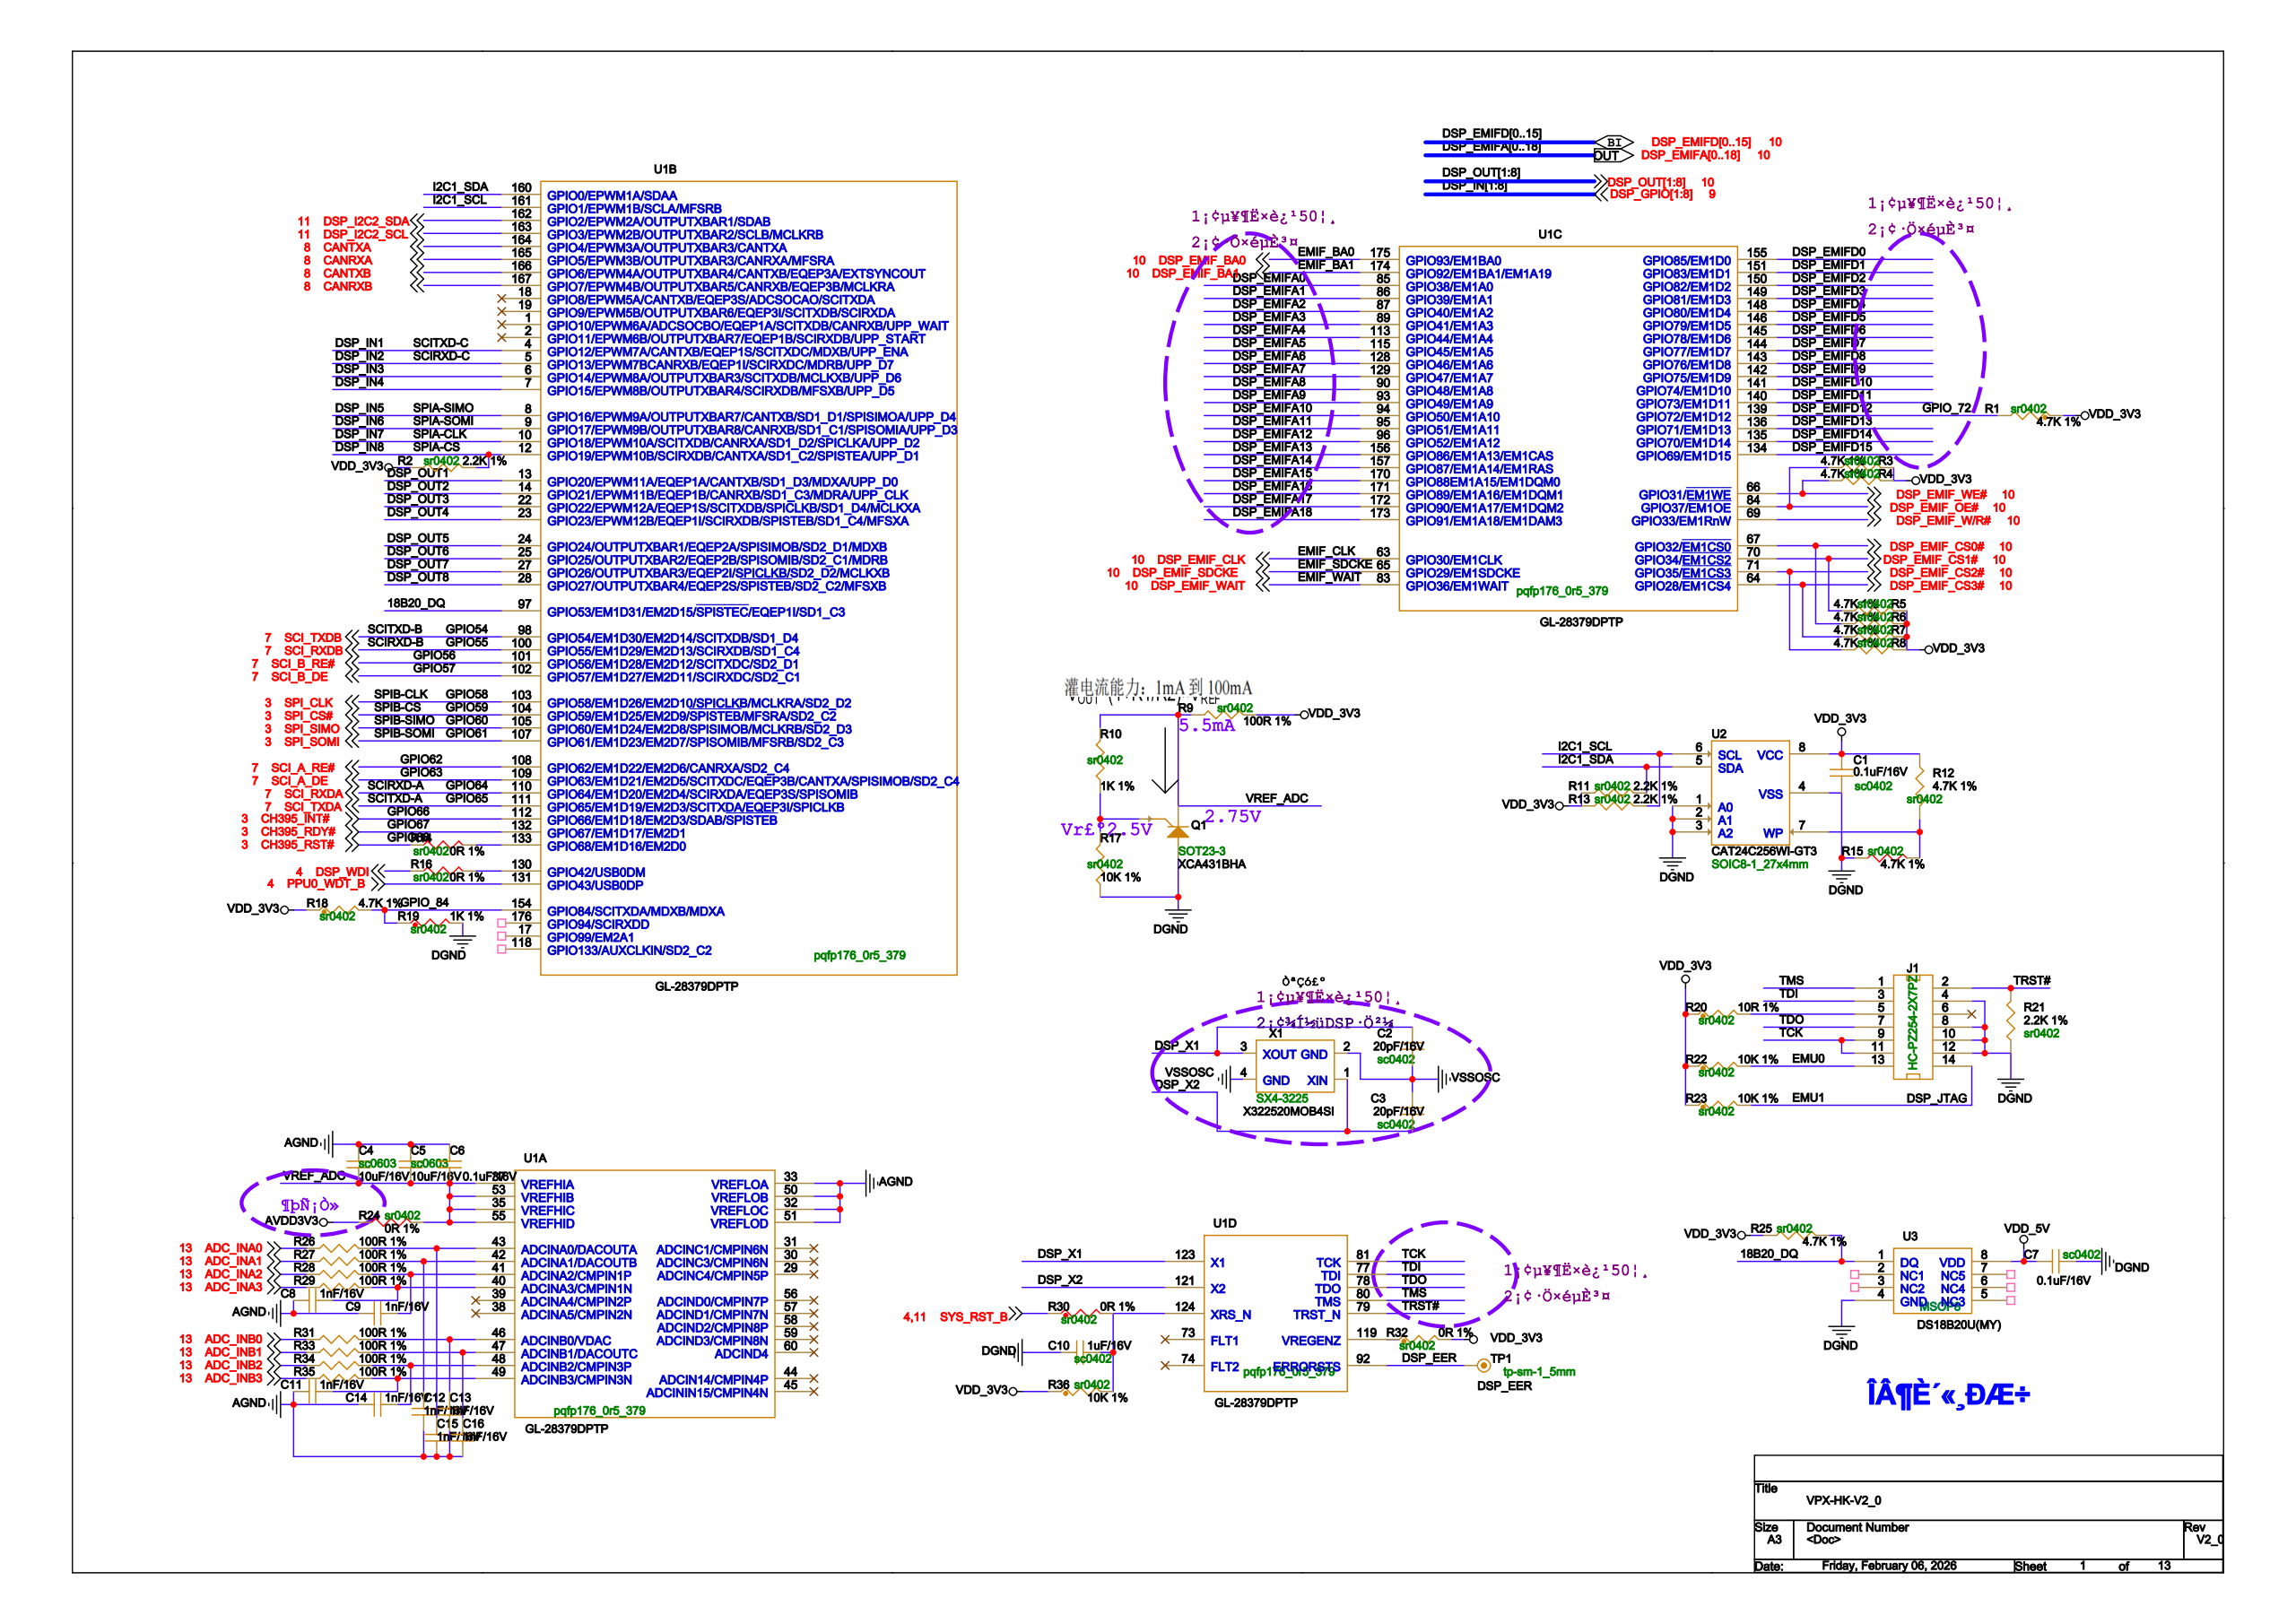Circuit board | Cadence Allegro | 598 parts | 541 nets | one sheet of the schematic
Parts on this sheet (reference | value | footprint):
C2 | 20pF/16V | SC0402
C3 | 20pF/16V | SC0402
C4 | 10uF/16V | SC0603
C5 | 10uF/16V | SC0603
C6 | 0.1uF/16V | SC0402
C8 | 1nF/16V | SC0402
C9 | 1nF/16V | SC0402
C10 | 1uF/16V | SC0402
C11 | 1nF/16V | SC0402
C13 | 1nF/16V | SC0402
C14 | 1nF/16V | SC0402
C15 | 1nF/16V | SC0402
C16 | 1nF/16V | SC0402
J1 | DSP_JTAG | HC-PZ254-2X7PZ
Q1 | XCA431BHA | SOT23-3
R1 | 4.7K 1% | SR0402
R2 | 2.2K 1% | SR0402
R9 | 100R 1% | SR0402
R10 | 1K 1% | SR0402
R11 | 2.2K 1% | SR0402
R12 | 4.7K 1% | SR0402
R13 | 2.2K 1% | SR0402
R14 | 0R 1% | SR0402
R15 | 4.7K 1% | SR0402
R16 | 0R 1% | SR0402
R17 | 10K 1% | SR0402
R18 | 4.7K 1% | SR0402
R19 | 1K 1% | SR0402
R20 | 10R 1% | SR0402
R21 | 2.2K 1% | SR0402
R22 | 10K 1% | SR0402
R23 | 10K 1% | SR0402
R24 | 0R 1% | SR0402
R25 | 4.7K 1% | SR0402
R26 | 100R 1% | SR0402
R27 | 100R 1% | SR0402
R28 | 100R 1% | SR0402
R29 | 100R 1% | SR0402
R30 | 0R 1% | SR0402
R31 | 100R 1% | SR0402
R32 | 0R 1% | SR0402
R33 | 100R 1% | SR0402
R34 | 100R 1% | SR0402
R35 | 100R 1% | SR0402
R36 | 10K 1% | SR0402
TP1 | DSP_EER | TP-SM-1_5MM
U1 | GL-28379DPTP | PQFP176_0R5_379
U2 | CAT24C256WI-GT3 | SOIC8-1_27X4MM
U3 | DS18B20U(MY) | MSOP8
X1 | X322520MOB4SI | SX4-3225
Nets of these parts (net: part-pin ...):
DGND: C10-1 J1-4 J1-8 J1-10 J1-12 Q1-3 R15-2 R17-1 R19-2 R21-2 U2-1 U2-2 U2-3 U2-4 U3-4
VDD_5V: U3-8
DSP_GPIO8: R2-2 U1-12
DSP_OUT7: U1-27
DSP_OUT8: U1-28
DSP_EMIF_CS2#: U1-71
DSP_EMIF_CS3#: U1-64
DSP_EMIF_CS1#: U1-70
DSP_EMIF_CS0#: U1-67
DSP_EMIF_WAIT: U1-83
DSP_EMIF_SDCKE: U1-65
DSP_EMIF_CLK: U1-63
DSP_EMIF_W/R#: U1-69
DSP_EMIF_OE#: U1-84
DSP_EMIF_WE#: U1-66
DSP_EMIF_BA1: U1-174
DSP_EMIF_BA0: U1-175
DSP_EMIFA18: U1-173
DSP_EMIFA17: U1-172
DSP_EMIFA16: U1-171
DSP_EMIFA15: U1-170
DSP_EMIFA14: U1-157
DSP_EMIFA13: U1-156
DSP_EMIFA12: U1-96
DSP_EMIFA11: U1-95
DSP_EMIFA10: U1-94
DSP_EMIFA9: U1-93
DSP_EMIFA8: U1-90
DSP_EMIFA7: U1-129
DSP_EMIFA6: U1-128
DSP_EMIFA5: U1-115
DSP_EMIFA4: U1-113
DSP_EMIFA3: U1-89
DSP_EMIFA2: U1-87
DSP_EMIFA1: U1-86
DSP_EMIFA0: U1-85
DSP_OUT5: U1-24
DSP_OUT6: U1-25
VDD_3V3: R1-1 R2-1 R9-2 R11-1 R12-2 R13-1 R18-1 R20-1 R22-1 R23-1 R25-1 R32-2 R36-1 U2-8
N33091267: C10-2 R30-2 R36-2 U1-124
AGND: C4-2 C5-2 C6-2 C8-1 C9-1 C11-1 C13-1 C14-1 C15-1 C16-1 U1-32 U1-33 U1-50 U1-51
N33522481: C11-2 R35-2 U1-49
N33522343: R27-2 U1-42
N33522484: C13-2 R31-2 U1-46
N33522478: C14-2 R34-2 U1-48
N33522280: C15-2 R26-2 U1-43
N33522487: C16-2 R33-2 U1-47
N33522388: C8-2 R29-2 U1-40
N33522385: C9-2 R28-2 U1-41
VSSOSC: C2-2 C3-1 X1-2 X1-4
AVDD3V3: R24-2
CH395_RST#: R14-1
N33617240: R14-2 U1-133
DSP_WDI: R16-1
N33616037: R16-2 U1-130
VREF_ADC: C4-1 C5-1 C6-1 Q1-2 R9-1 R10-2 R24-1 U1-35 U1-37 U1-53 U1-55
18B20_DQ: R25-2 U3-1 U1-97
SYS_RST_B: R30-1
DSP_X1: C2-1 X1-3 U1-123
DSP_X2: C3-2 X1-1 U1-121
TMS: J1-1 U1-80
EMU1: J1-14 R23-2
TDI: J1-3 U1-77
N32268466: J1-5 R20-2
TDO: J1-7 U1-78
TCK: J1-9 J1-11 U1-81
EMU0: J1-13 R22-2
TRST#: J1-2 R21-1 U1-79
ADC_INA0: R26-1
ADC_INB0: R31-1
ADC_INA1: R27-1
ADC_INB1: R33-1
ADC_INA2: R28-1
ADC_INB2: R34-1
ADC_INA3: R29-1
ADC_INB3: R35-1
N33553932: Q1-1 R10-1 R17-2
SPI_SOMI: U1-107
DSP_EMIFD12: R1-2 U1-139
GPIO_84: R18-2 R19-1 U1-154
DSP_I2C2_SCL: U1-163
I2C1_SDA: R11-2 U2-5 U1-160
I2C1_SCL: R13-2 U2-6 U1-161
DSP_I2C2_SDA: U1-162
N32267709: R12-1 R15-1 U2-7
CANTXA: U1-164
CANRXA: U1-165
CANTXB: U1-166
CANRXB: U1-167
SCI_B_RE#: U1-101
SCI_B_DE: U1-102
SCI_A_RE#: U1-108
SCI_A_DE: U1-109
DSP_EMIFD15: U1-134
DSP_OUT4: U1-23
DSP_EMIFD0: U1-155
DSP_EMIFD7: U1-144
DSP_EMIFD1: U1-151
DSP_EMIFD2: U1-150
DSP_EMIFD3: U1-149
DSP_EMIFD4: U1-148
DSP_EMIFD5: U1-146
DSP_EMIFD6: U1-145
DSP_EMIFD8: U1-143
DSP_EMIFD9: U1-142
DSP_EMIFD10: U1-141
DSP_EMIFD11: U1-140
DSP_EMIFD13: U1-136
DSP_EMIFD14: U1-135
DSP_OUT1: U1-13
DSP_OUT2: U1-14
DSP_OUT3: U1-22
DSP_EER: TP1-1 U1-92
PPU0_WDT_B: U1-131
SCI_TXDB: U1-98
SCI_RXDB: U1-100
SPI_CLK: U1-103
SPI_CS#: U1-104
SPI_SIMO: U1-105
SCI_RXDA: U1-110
SCI_TXDA: U1-111
CH395_INT#: U1-112
CH395_RDY#: U1-132
N33073148: R32-1 U1-119